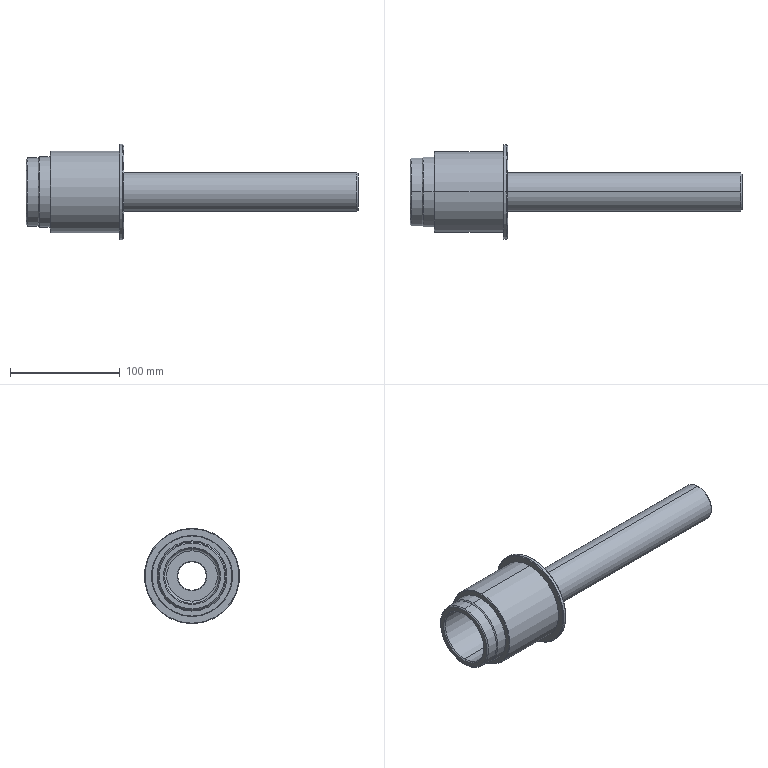Part | SolidWorks | features BaseBody 2 | 2 solids | 68 faces | box 302.5 x 87 x 87 mm | volume 330300 mm3 | cylinder 28 | cone 26 | plane 12 | torus 2 | commonest cylinder face diameters 35 x6 32 x4 34 x4 26 x2 27 x2 50 x2